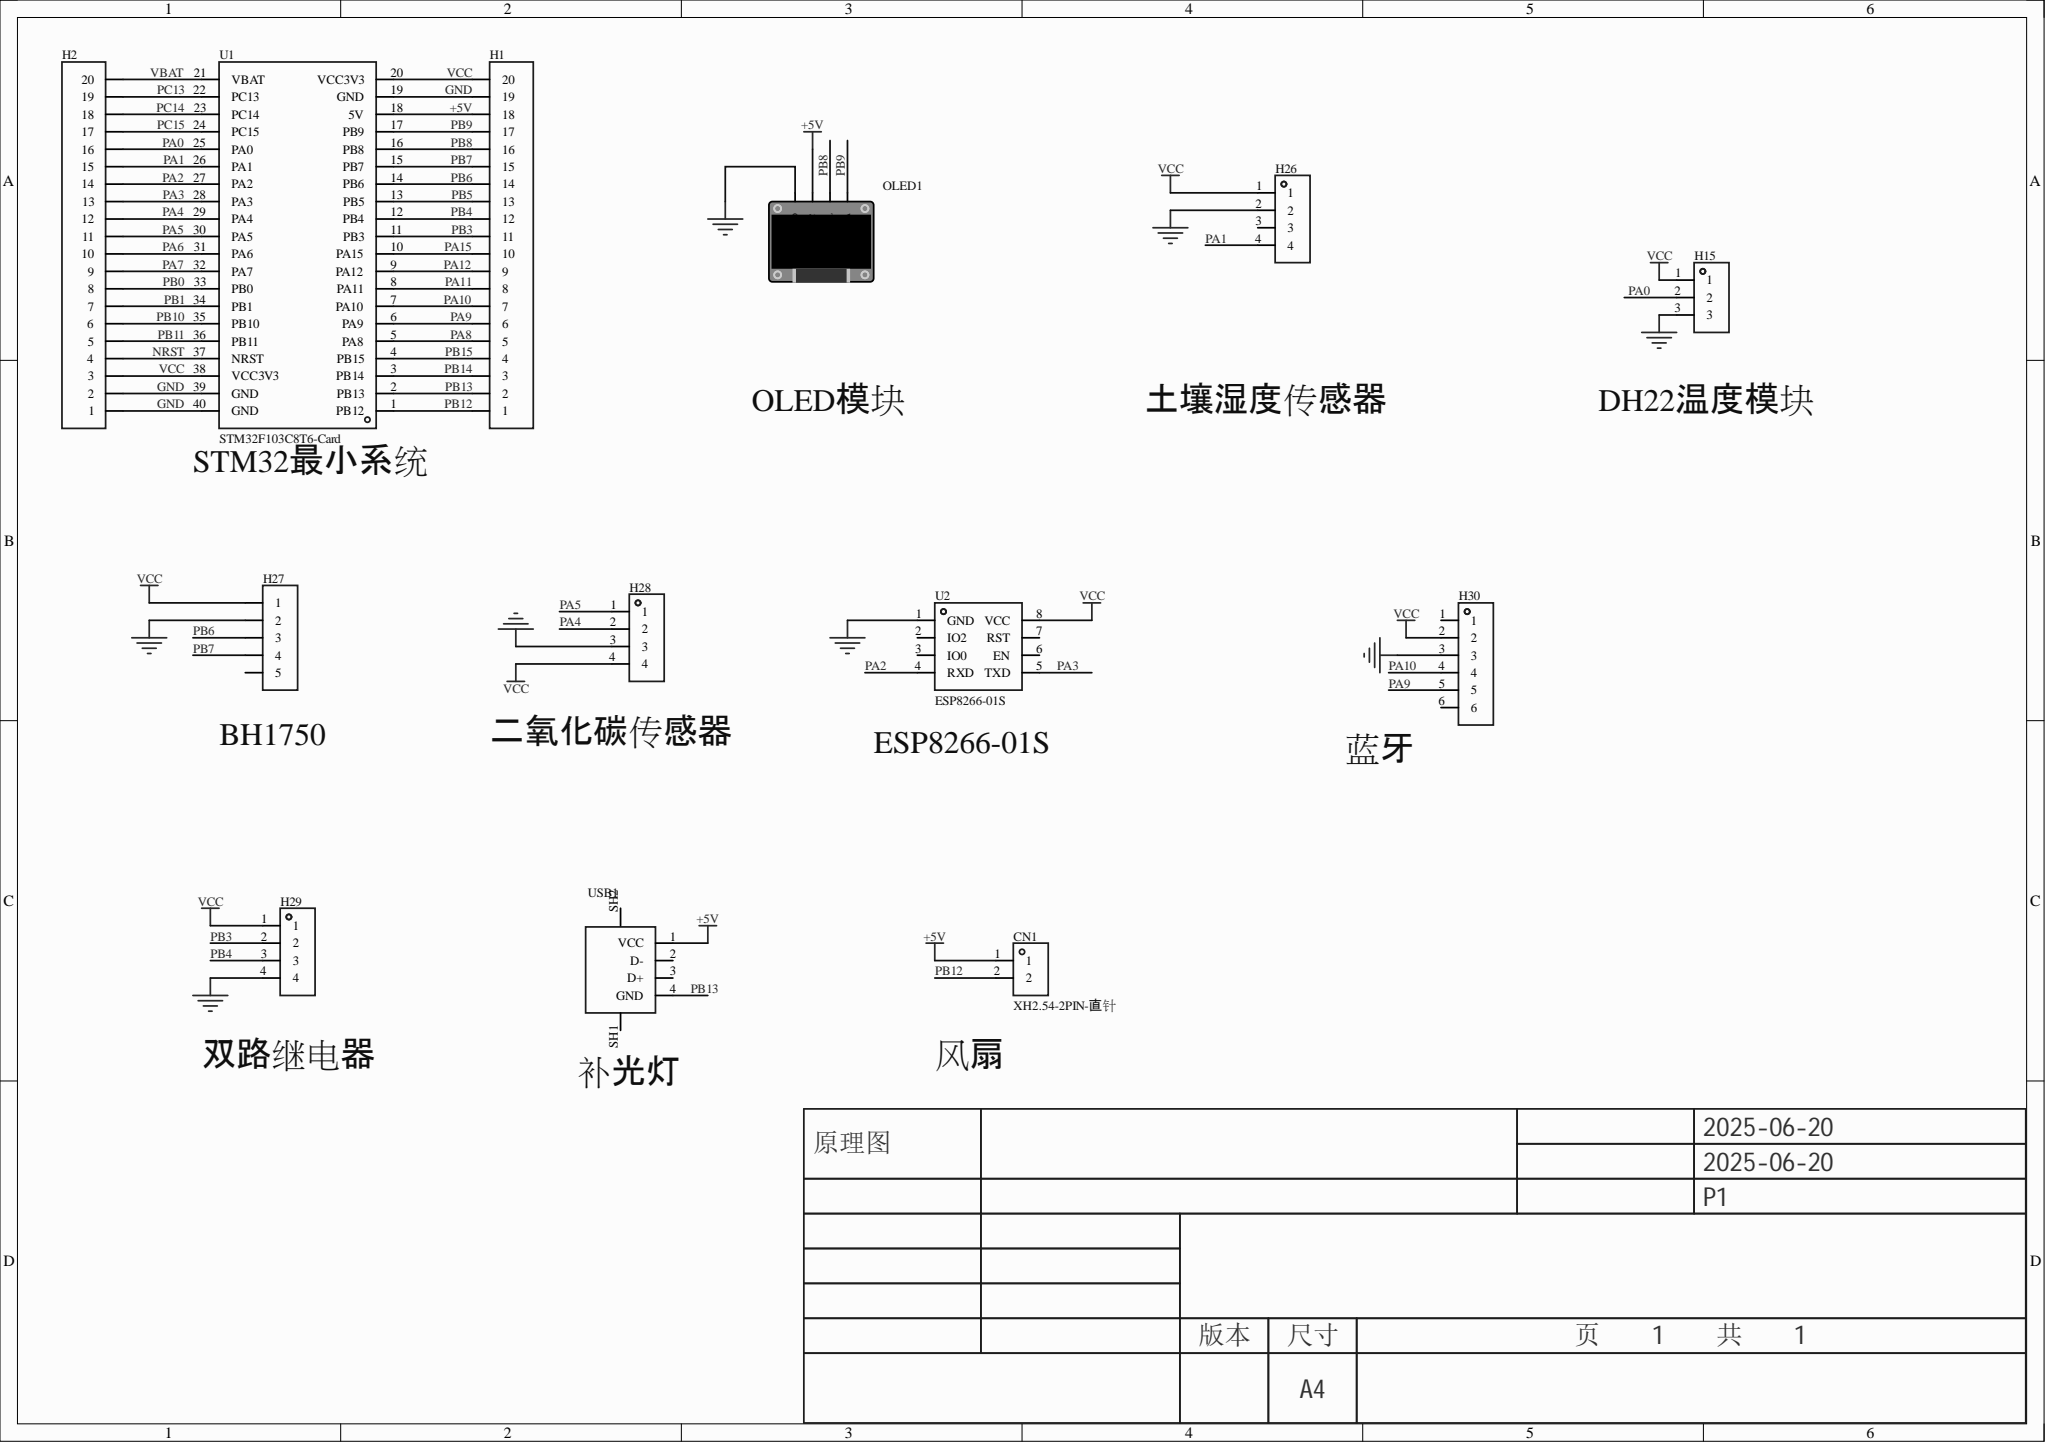Circuit board | Altium Designer | 13 parts | 37 nets
Bill of materials:
Comment,Description,Designator,Footprint,LibRef,Quantity
"XH2.54-2PIN-直针","","CN1","CONN-TH_XH2.54-2P","XH2.54-2PIN-直针","1"
"","","H1, H2","HDR-TH_20P-P2.54-V-F","HDR-F_2.54_1x20P","2"
"","","H15","HDR-TH_3P-P2.54-V-F","HDR-F_2.54_1x3P","1"
"","","H26, H28, H29","HDR-TH_4P-P2.54-V-F","HDR-F_2.54_1x4P","3"
"","","H27","HDR-TH_5P-P2.54-V-F","HDR-F_2.54_1x5P","1"
"","","H30","HDR-TH_6P-P2.54-V-F","HDR-F_2.54_1x6P","1"
"","","OLED1","0.96OLED_4P","0.96OLED模块_4P","1"
"STM32F103C8T6-Card","","U1","CONN-TH_L53.3-W22.9_STM32F103C8T6-CARD","STM32F103C8T6-Card","1"
"ESP8266-01S","","U2","WIFIM-TH_ESP8266-01S","ESP8266-01S","1"
"","","USB1","USB_ Type-A","USB_ Type-A","1"
Netlist (Protel format):
[
CN1
CONN-TH_XH2.54-2P
XH2.54-2PIN-直针



]
[
H1
HDR-TH_20P-P2.54-V-F




]
[
H2
HDR-TH_20P-P2.54-V-F




]
[
H15
HDR-TH_3P-P2.54-V-F




]
[
H26
HDR-TH_4P-P2.54-V-F




]
[
H27
HDR-TH_5P-P2.54-V-F




]
[
H28
HDR-TH_4P-P2.54-V-F




]
[
H29
HDR-TH_4P-P2.54-V-F




]
[
H30
HDR-TH_6P-P2.54-V-F




]
[
OLED1
0.96OLED_4P




]
[
U1
CONN-TH_L53.3-W22.9_STM32F103C8T6-CARD
STM32F103C8T6-Card



]
[
U2
WIFIM-TH_ESP8266-01S
ESP8266-01S



]
[
USB1
USB_ Type-A




]
(
VCC
H1-20
H2-3
H15-1
H26-1
H27-1
H28-4
H29-1
H30-2
U1-20
U1-38
U2-8
)
(
VBAT
H2-20
U1-21
)
(
PC15
H2-17
U1-24
)
(
PC14
H2-18
U1-23
)
(
PC13
H2-19
U1-22
)
(
PB15
H1-4
U1-4
)
(
PB14
H1-3
U1-3
)
(
PB13
H1-2
U1-2
USB1-4
)
(
PB12
CN1-2
H1-1
U1-1
)
(
PB11
H2-5
U1-36
)
(
PB10
H2-6
U1-35
)
(
PB9
H1-17
OLED1-4
U1-17
)
(
PB8
H1-16
OLED1-3
U1-16
)
(
PB7
H1-15
H27-4
U1-15
)
(
PB6
H1-14
H27-3
U1-14
)
(
PB5
H1-13
U1-13
)
(
PB4
H1-12
H29-3
U1-12
)
(
PB3
H1-11
H29-2
U1-11
)
(
PB1
H2-7
U1-34
)
(
PB0
H2-8
U1-33
)
(
PA15
H1-10
U1-10
)
(
PA12
H1-9
U1-9
)
(
PA11
H1-8
U1-8
)
(
PA10
H1-7
H30-4
U1-7
)
(
PA9
H1-6
H30-5
U1-6
)
(
PA8
H1-5
U1-5
)
(
PA7
H2-9
U1-32
)
(
PA6
H2-10
U1-31
)
(
PA5
H2-11
H28-1
U1-30
)
(
PA4
H2-12
H28-2
U1-29
)
(
PA3
H2-13
U1-28
U2-5
)
(
PA2
H2-14
U1-27
U2-4
)
(
PA1
H2-15
H26-4
U1-26
)
(
PA0
H2-16
H15-2
U1-25
)
(
NRST
H2-4
U1-37
)
(
GND
H1-19
H2-1
H2-2
H15-3
H26-2
H27-2
H28-3
H29-4
H30-3
OLED1-1
U1-19
U1-39
U1-40
U2-1
)
(
+5V
CN1-1
H1-18
OLED1-2
U1-18
USB1-1
)